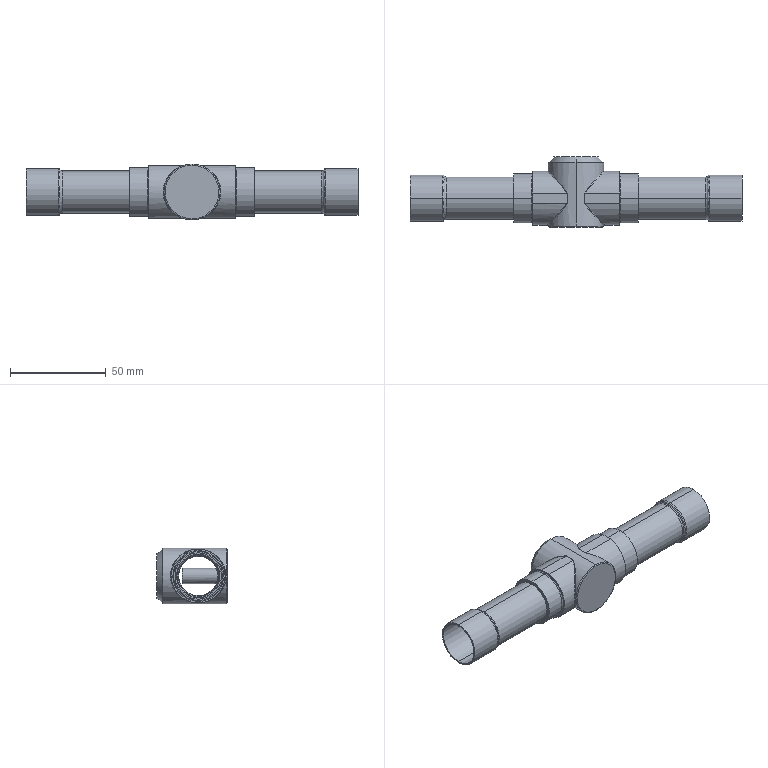Part | STEP file | SGN22S-sight glass | 4 solids | 107 faces | box 173 x 36.5 x 29 mm | volume 27166 mm3 | cylinder 47 | spline 26 | plane 22 | cone 12 | commonest cylinder face diameters 22 x6 13 x5 1 x4 20.4 x4 22.6 x4 24.2 x4